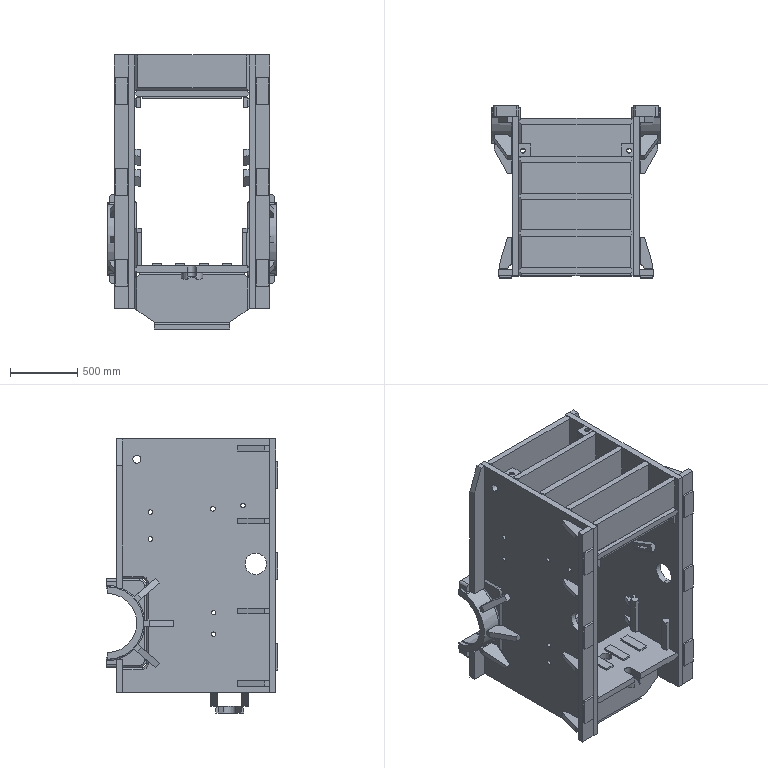Part | SolidWorks | features ReferencePattern 27, MirrorCompFeat 8, LocalCirPattern 2, LocalLPattern 1 | 69 solids | 959 faces | box 1256 x 1280 x 2040 mm | volume 426098294 mm3 | plane 754 | cylinder 155 | cone 32 | torus 12 | spline 4 | sphere 2 | commonest cylinder face diameters 25 x16 26.5 x16 35 x16 80 x16 20 x14 33 x8